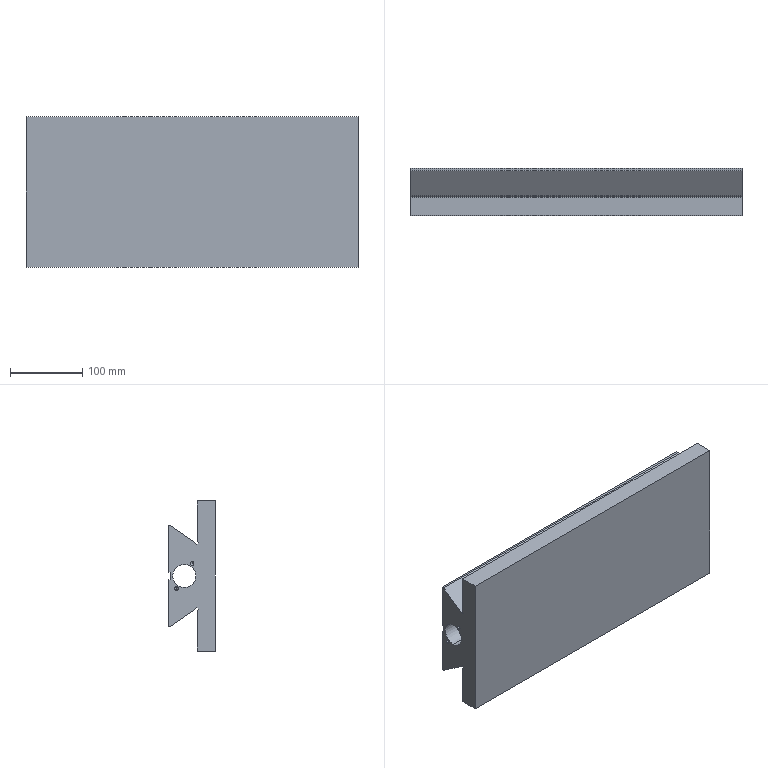Part | SolidWorks | features HoleWzd 2, ICE 2, Extrusion 1 | 1 solid | 50 faces | box 460 x 65 x 208 mm | volume 2873853 mm3 | plane 30 | cylinder 12 | cone 8 | commonest cylinder face diameters 5 x8 32 x4
STEP:
#1=CARTESIAN_POINT('',(17.,19.747,14.954));
#2=VERTEX_POINT('',#1);
#3=CARTESIAN_POINT('',(17.,19.747,19.954));
#4=VERTEX_POINT('',#3);
#5=CARTESIAN_POINT('',(17.,19.747,17.454));
#6=DIRECTION('',(-1.,0.,0.));
#7=DIRECTION('',(0.,0.,1.));
#8=AXIS2_PLACEMENT_3D('',#5,#6,#7);
#9=CIRCLE('',#8,2.5);
#10=EDGE_CURVE('',#2,#4,#9,.T.);
#11=ORIENTED_EDGE('',*,*,#10,.F.);
#12=CARTESIAN_POINT('',(0.,19.747,14.954));
#13=VERTEX_POINT('',#12);
#14=CARTESIAN_POINT('',(0.,19.747,14.954));
#15=DIRECTION('',(-1.,0.,0.));
#16=VECTOR('',#15,1000.);
#17=LINE('',#14,#16);
#18=EDGE_CURVE('',#2,#13,#17,.T.);
#19=ORIENTED_EDGE('',*,*,#18,.T.);
#20=CARTESIAN_POINT('',(0.,19.747,19.954));
#21=VERTEX_POINT('',#20);
#22=CARTESIAN_POINT('',(0.,19.747,17.454));
#23=DIRECTION('',(-1.,0.,0.));
#24=DIRECTION('',(0.,0.,1.));
#25=AXIS2_PLACEMENT_3D('',#22,#23,#24);
#26=CIRCLE('',#25,2.5);
#27=EDGE_CURVE('',#13,#21,#26,.T.);
#28=ORIENTED_EDGE('',*,*,#27,.T.);
#29=CARTESIAN_POINT('',(0.,19.747,19.954));
#30=DIRECTION('',(-1.,0.,0.));
#31=VECTOR('',#30,1000.);
#32=LINE('',#29,#31);
#33=EDGE_CURVE('',#4,#21,#32,.T.);
#34=ORIENTED_EDGE('',*,*,#33,.F.);
#35=EDGE_LOOP('',(#11,#19,#28,#34));
#36=FACE_OUTER_BOUND('',#35,.T.);
#37=CARTESIAN_POINT('',(0.,19.747,17.454));
#38=DIRECTION('',(-1.,0.,0.));
#39=DIRECTION('',(0.,0.,1.));
#40=AXIS2_PLACEMENT_3D('',#37,#38,#39);
#41=CYLINDRICAL_SURFACE('',#40,2.5);
#42=ADVANCED_FACE('',(#36),#41,.F.);
#43=CARTESIAN_POINT('',(18.502,19.747,17.454));
#44=VERTEX_POINT('',#43);
#45=CARTESIAN_POINT('',(17.,19.747,19.954));
#46=DIRECTION('',(-0.515,0.,0.8572));
#47=VECTOR('',#46,1000.);
#48=LINE('',#45,#47);
#49=EDGE_CURVE('',#44,#4,#48,.T.);
#50=ORIENTED_EDGE('',*,*,#49,.F.);
#51=CARTESIAN_POINT('',(17.,19.747,14.954));
#52=DIRECTION('',(-0.515,0.,-0.8572));
#53=VECTOR('',#52,1000.);
#54=LINE('',#51,#53);
#55=EDGE_CURVE('',#44,#2,#54,.T.);
#56=ORIENTED_EDGE('',*,*,#55,.T.);
#57=ORIENTED_EDGE('',*,*,#10,.T.);
#58=EDGE_LOOP('',(#50,#56,#57));
#59=FACE_OUTER_BOUND('',#58,.T.);
#60=CARTESIAN_POINT('',(17.,19.747,17.454));
#61=DIRECTION('',(-1.,0.,0.));
#62=DIRECTION('',(0.,0.,1.));
#63=AXIS2_PLACEMENT_3D('',#60,#61,#62);
#64=CONICAL_SURFACE('',#63,2.5,1.03);
#65=ADVANCED_FACE('',(#59),#64,.F.);
#66=CARTESIAN_POINT('',(17.,41.253,-19.954));
#67=VERTEX_POINT('',#66);
#68=CARTESIAN_POINT('',(17.,41.253,-14.954));
#69=VERTEX_POINT('',#68);
#70=CARTESIAN_POINT('',(17.,41.253,-17.454));
#71=DIRECTION('',(-1.,0.,0.));
#72=DIRECTION('',(0.,0.,1.));
#73=AXIS2_PLACEMENT_3D('',#70,#71,#72);
#74=CIRCLE('',#73,2.5);
#75=EDGE_CURVE('',#67,#69,#74,.T.);
#76=ORIENTED_EDGE('',*,*,#75,.F.);
#77=CARTESIAN_POINT('',(0.,41.253,-19.954));
#78=VERTEX_POINT('',#77);
#79=CARTESIAN_POINT('',(0.,41.253,-19.954));
#80=DIRECTION('',(-1.,0.,0.));
#81=VECTOR('',#80,1000.);
#82=LINE('',#79,#81);
#83=EDGE_CURVE('',#67,#78,#82,.T.);
#84=ORIENTED_EDGE('',*,*,#83,.T.);
#85=CARTESIAN_POINT('',(0.,41.253,-14.954));
#86=VERTEX_POINT('',#85);
#87=CARTESIAN_POINT('',(0.,41.253,-17.454));
#88=DIRECTION('',(-1.,0.,0.));
#89=DIRECTION('',(0.,0.,1.));
#90=AXIS2_PLACEMENT_3D('',#87,#88,#89);
#91=CIRCLE('',#90,2.5);
#92=EDGE_CURVE('',#78,#86,#91,.T.);
#93=ORIENTED_EDGE('',*,*,#92,.T.);
#94=CARTESIAN_POINT('',(0.,41.253,-14.954));
#95=DIRECTION('',(-1.,0.,0.));
#96=VECTOR('',#95,1000.);
#97=LINE('',#94,#96);
#98=EDGE_CURVE('',#69,#86,#97,.T.);
#99=ORIENTED_EDGE('',*,*,#98,.F.);
#100=EDGE_LOOP('',(#76,#84,#93,#99));
#101=FACE_OUTER_BOUND('',#100,.T.);
#102=CARTESIAN_POINT('',(0.,41.253,-17.454));
#103=DIRECTION('',(-1.,0.,0.));
#104=DIRECTION('',(0.,0.,1.));
#105=AXIS2_PLACEMENT_3D('',#102,#103,#104);
#106=CYLINDRICAL_SURFACE('',#105,2.5);
#107=ADVANCED_FACE('',(#101),#106,.F.);
#108=CARTESIAN_POINT('',(18.502,41.253,-17.454));
#109=VERTEX_POINT('',#108);
#110=CARTESIAN_POINT('',(17.,41.253,-14.954));
#111=DIRECTION('',(-0.515,0.,0.8572));
#112=VECTOR('',#111,1000.);
#113=LINE('',#110,#112);
#114=EDGE_CURVE('',#109,#69,#113,.T.);
#115=ORIENTED_EDGE('',*,*,#114,.F.);
#116=CARTESIAN_POINT('',(17.,41.253,-19.954));
#117=DIRECTION('',(-0.515,0.,-0.8572));
#118=VECTOR('',#117,1000.);
#119=LINE('',#116,#118);
#120=EDGE_CURVE('',#109,#67,#119,.T.);
#121=ORIENTED_EDGE('',*,*,#120,.T.);
#122=ORIENTED_EDGE('',*,*,#75,.T.);
#123=EDGE_LOOP('',(#115,#121,#122));
#124=FACE_OUTER_BOUND('',#123,.T.);
#125=CARTESIAN_POINT('',(17.,41.253,-17.454));
#126=DIRECTION('',(-1.,0.,0.));
#127=DIRECTION('',(0.,0.,1.));
#128=AXIS2_PLACEMENT_3D('',#125,#126,#127);
#129=CONICAL_SURFACE('',#128,2.5,1.03);
#130=ADVANCED_FACE('',(#124),#129,.F.);
#131=CARTESIAN_POINT('',(443.,30.5,23.));
#132=VERTEX_POINT('',#131);
#133=CARTESIAN_POINT('',(443.,30.5,18.));
#134=VERTEX_POINT('',#133);
#135=CARTESIAN_POINT('',(443.,30.5,20.5));
#136=DIRECTION('',(1.,0.,0.));
#137=DIRECTION('',(0.,0.,-1.));
#138=AXIS2_PLACEMENT_3D('',#135,#136,#137);
#139=CIRCLE('',#138,2.5);
#140=EDGE_CURVE('',#132,#134,#139,.T.);
#141=ORIENTED_EDGE('',*,*,#140,.F.);
#142=CARTESIAN_POINT('',(460.,30.5,23.));
#143=VERTEX_POINT('',#142);
#144=CARTESIAN_POINT('',(460.,30.5,23.));
#145=DIRECTION('',(1.,0.,0.));
#146=VECTOR('',#145,1000.);
#147=LINE('',#144,#146);
#148=EDGE_CURVE('',#132,#143,#147,.T.);
#149=ORIENTED_EDGE('',*,*,#148,.T.);
#150=CARTESIAN_POINT('',(460.,30.5,18.));
#151=VERTEX_POINT('',#150);
#152=CARTESIAN_POINT('',(460.,30.5,20.5));
#153=DIRECTION('',(1.,0.,0.));
#154=DIRECTION('',(0.,0.,-1.));
#155=AXIS2_PLACEMENT_3D('',#152,#153,#154);
#156=CIRCLE('',#155,2.5);
#157=EDGE_CURVE('',#143,#151,#156,.T.);
#158=ORIENTED_EDGE('',*,*,#157,.T.);
#159=CARTESIAN_POINT('',(460.,30.5,18.));
#160=DIRECTION('',(1.,0.,0.));
#161=VECTOR('',#160,1000.);
#162=LINE('',#159,#161);
#163=EDGE_CURVE('',#134,#151,#162,.T.);
#164=ORIENTED_EDGE('',*,*,#163,.F.);
#165=EDGE_LOOP('',(#141,#149,#158,#164));
#166=FACE_OUTER_BOUND('',#165,.T.);
#167=CARTESIAN_POINT('',(460.,30.5,20.5));
#168=DIRECTION('',(1.,0.,0.));
#169=DIRECTION('',(0.,0.,-1.));
#170=AXIS2_PLACEMENT_3D('',#167,#168,#169);
#171=CYLINDRICAL_SURFACE('',#170,2.5);
#172=ADVANCED_FACE('',(#166),#171,.F.);
#173=CARTESIAN_POINT('',(441.498,30.5,20.5));
#174=VERTEX_POINT('',#173);
#175=CARTESIAN_POINT('',(443.,30.5,18.));
#176=DIRECTION('',(0.515,0.,-0.8572));
#177=VECTOR('',#176,1000.);
#178=LINE('',#175,#177);
#179=EDGE_CURVE('',#174,#134,#178,.T.);
#180=ORIENTED_EDGE('',*,*,#179,.F.);
#181=CARTESIAN_POINT('',(443.,30.5,23.));
#182=DIRECTION('',(0.515,0.,0.8572));
#183=VECTOR('',#182,1000.);
#184=LINE('',#181,#183);
#185=EDGE_CURVE('',#174,#132,#184,.T.);
#186=ORIENTED_EDGE('',*,*,#185,.T.);
#187=ORIENTED_EDGE('',*,*,#140,.T.);
#188=EDGE_LOOP('',(#180,#186,#187));
#189=FACE_OUTER_BOUND('',#188,.T.);
#190=CARTESIAN_POINT('',(443.,30.5,20.5));
#191=DIRECTION('',(1.,0.,0.));
#192=DIRECTION('',(0.,0.,-1.));
#193=AXIS2_PLACEMENT_3D('',#190,#191,#192);
#194=CONICAL_SURFACE('',#193,2.5,1.03);
#195=ADVANCED_FACE('',(#189),#194,.F.);
#196=CARTESIAN_POINT('',(443.,30.5,-18.));
#197=VERTEX_POINT('',#196);
#198=CARTESIAN_POINT('',(443.,30.5,-23.));
#199=VERTEX_POINT('',#198);
#200=CARTESIAN_POINT('',(443.,30.5,-20.5));
#201=DIRECTION('',(1.,0.,0.));
#202=DIRECTION('',(0.,0.,-1.));
#203=AXIS2_PLACEMENT_3D('',#200,#201,#202);
#204=CIRCLE('',#203,2.5);
#205=EDGE_CURVE('',#197,#199,#204,.T.);
#206=ORIENTED_EDGE('',*,*,#205,.F.);
#207=CARTESIAN_POINT('',(460.,30.5,-18.));
#208=VERTEX_POINT('',#207);
#209=CARTESIAN_POINT('',(460.,30.5,-18.));
#210=DIRECTION('',(1.,0.,0.));
#211=VECTOR('',#210,1000.);
#212=LINE('',#209,#211);
#213=EDGE_CURVE('',#197,#208,#212,.T.);
#214=ORIENTED_EDGE('',*,*,#213,.T.);
#215=CARTESIAN_POINT('',(460.,30.5,-23.));
#216=VERTEX_POINT('',#215);
#217=CARTESIAN_POINT('',(460.,30.5,-20.5));
#218=DIRECTION('',(1.,0.,0.));
#219=DIRECTION('',(0.,0.,-1.));
#220=AXIS2_PLACEMENT_3D('',#217,#218,#219);
#221=CIRCLE('',#220,2.5);
#222=EDGE_CURVE('',#208,#216,#221,.T.);
#223=ORIENTED_EDGE('',*,*,#222,.T.);
#224=CARTESIAN_POINT('',(460.,30.5,-23.));
#225=DIRECTION('',(1.,0.,0.));
#226=VECTOR('',#225,1000.);
#227=LINE('',#224,#226);
#228=EDGE_CURVE('',#199,#216,#227,.T.);
#229=ORIENTED_EDGE('',*,*,#228,.F.);
#230=EDGE_LOOP('',(#206,#214,#223,#229));
#231=FACE_OUTER_BOUND('',#230,.T.);
#232=CARTESIAN_POINT('',(460.,30.5,-20.5));
#233=DIRECTION('',(1.,0.,0.));
#234=DIRECTION('',(0.,0.,-1.));
#235=AXIS2_PLACEMENT_3D('',#232,#233,#234);
#236=CYLINDRICAL_SURFACE('',#235,2.5);
#237=ADVANCED_FACE('',(#231),#236,.F.);
#238=CARTESIAN_POINT('',(441.498,30.5,-20.5));
#239=VERTEX_POINT('',#238);
#240=CARTESIAN_POINT('',(443.,30.5,-23.));
#241=DIRECTION('',(0.515,0.,-0.8572));
#242=VECTOR('',#241,1000.);
#243=LINE('',#240,#242);
#244=EDGE_CURVE('',#239,#199,#243,.T.);
#245=ORIENTED_EDGE('',*,*,#244,.F.);
#246=CARTESIAN_POINT('',(443.,30.5,-18.));
#247=DIRECTION('',(0.515,0.,0.8572));
#248=VECTOR('',#247,1000.);
#249=LINE('',#246,#248);
#250=EDGE_CURVE('',#239,#197,#249,.T.);
#251=ORIENTED_EDGE('',*,*,#250,.T.);
#252=ORIENTED_EDGE('',*,*,#205,.T.);
#253=EDGE_LOOP('',(#245,#251,#252));
#254=FACE_OUTER_BOUND('',#253,.T.);
#255=CARTESIAN_POINT('',(443.,30.5,-20.5));
#256=DIRECTION('',(1.,0.,0.));
#257=DIRECTION('',(0.,0.,-1.));
#258=AXIS2_PLACEMENT_3D('',#255,#256,#257);
#259=CONICAL_SURFACE('',#258,2.5,1.03);
#260=ADVANCED_FACE('',(#254),#259,.F.);
#261=CARTESIAN_POINT('',(430.,30.5,16.));
#262=VERTEX_POINT('',#261);
#263=CARTESIAN_POINT('',(430.,30.5,-16.));
#264=VERTEX_POINT('',#263);
#265=CARTESIAN_POINT('',(430.,30.5,0.));
#266=DIRECTION('',(1.,0.,0.));
#267=DIRECTION('',(0.,0.,-1.));
#268=AXIS2_PLACEMENT_3D('',#265,#266,#267);
#269=CIRCLE('',#268,16.);
#270=EDGE_CURVE('',#262,#264,#269,.T.);
#271=ORIENTED_EDGE('',*,*,#270,.F.);
#272=CARTESIAN_POINT('',(460.,30.5,16.));
#273=VERTEX_POINT('',#272);
#274=CARTESIAN_POINT('',(0.,30.5,16.));
#275=DIRECTION('',(1.,0.,0.));
#276=VECTOR('',#275,1000.);
#277=LINE('',#274,#276);
#278=EDGE_CURVE('',#262,#273,#277,.T.);
#279=ORIENTED_EDGE('',*,*,#278,.T.);
#280=CARTESIAN_POINT('',(460.,30.5,-16.));
#281=VERTEX_POINT('',#280);
#282=CARTESIAN_POINT('',(460.,30.5,0.));
#283=DIRECTION('',(1.,0.,0.));
#284=DIRECTION('',(0.,0.,-1.));
#285=AXIS2_PLACEMENT_3D('',#282,#283,#284);
#286=CIRCLE('',#285,16.);
#287=EDGE_CURVE('',#273,#281,#286,.T.);
#288=ORIENTED_EDGE('',*,*,#287,.T.);
#289=CARTESIAN_POINT('',(0.,30.5,-16.));
#290=DIRECTION('',(1.,0.,0.));
#291=VECTOR('',#290,1000.);
#292=LINE('',#289,#291);
#293=EDGE_CURVE('',#264,#281,#292,.T.);
#294=ORIENTED_EDGE('',*,*,#293,.F.);
#295=EDGE_LOOP('',(#271,#279,#288,#294));
#296=FACE_OUTER_BOUND('',#295,.T.);
#297=CARTESIAN_POINT('',(0.,30.5,0.));
#298=DIRECTION('',(1.,0.,0.));
#299=DIRECTION('',(0.,0.,-1.));
#300=AXIS2_PLACEMENT_3D('',#297,#298,#299);
#301=CYLINDRICAL_SURFACE('',#300,16.);
#302=ADVANCED_FACE('',(#296),#301,.F.);
#303=CARTESIAN_POINT('',(0.,30.5,16.));
#304=VERTEX_POINT('',#303);
#305=CARTESIAN_POINT('',(0.,30.5,-16.));
#306=VERTEX_POINT('',#305);
#307=CARTESIAN_POINT('',(0.,30.5,0.));
#308=DIRECTION('',(1.,0.,0.));
#309=DIRECTION('',(0.,0.,-1.));
#310=AXIS2_PLACEMENT_3D('',#307,#308,#309);
#311=CIRCLE('',#310,16.);
#312=EDGE_CURVE('',#304,#306,#311,.T.);
#313=ORIENTED_EDGE('',*,*,#312,.F.);
#314=CARTESIAN_POINT('',(30.,30.5,16.));
#315=VERTEX_POINT('',#314);
#316=CARTESIAN_POINT('',(0.,30.5,16.));
#317=DIRECTION('',(1.,0.,0.));
#318=VECTOR('',#317,1000.);
#319=LINE('',#316,#318);
#320=EDGE_CURVE('',#304,#315,#319,.T.);
#321=ORIENTED_EDGE('',*,*,#320,.T.);
#322=CARTESIAN_POINT('',(30.,30.5,-16.));
#323=VERTEX_POINT('',#322);
#324=CARTESIAN_POINT('',(30.,30.5,0.));
#325=DIRECTION('',(-1.,0.,0.));
#326=DIRECTION('',(0.,0.,1.));
#327=AXIS2_PLACEMENT_3D('',#324,#325,#326);
#328=CIRCLE('',#327,16.);
#329=EDGE_CURVE('',#323,#315,#328,.T.);
#330=ORIENTED_EDGE('',*,*,#329,.F.);
#331=CARTESIAN_POINT('',(0.,30.5,-16.));
#332=DIRECTION('',(1.,0.,0.));
#333=VECTOR('',#332,1000.);
#334=LINE('',#331,#333);
#335=EDGE_CURVE('',#306,#323,#334,.T.);
#336=ORIENTED_EDGE('',*,*,#335,.F.);
#337=EDGE_LOOP('',(#313,#321,#330,#336));
#338=FACE_OUTER_BOUND('',#337,.T.);
#339=CARTESIAN_POINT('',(0.,30.5,0.));
#340=DIRECTION('',(1.,0.,0.));
#341=DIRECTION('',(0.,0.,-1.));
#342=AXIS2_PLACEMENT_3D('',#339,#340,#341);
#343=CYLINDRICAL_SURFACE('',#342,16.);
#344=ADVANCED_FACE('',(#338),#343,.F.);
#345=CARTESIAN_POINT('',(460.,52.5,-5.));
#346=VERTEX_POINT('',#345);
#347=CARTESIAN_POINT('',(430.,52.5,-5.));
#348=VERTEX_POINT('',#347);
#349=CARTESIAN_POINT('',(460.,52.5,-5.));
#350=DIRECTION('',(-1.,0.,0.));
#351=VECTOR('',#350,1000.);
#352=LINE('',#349,#351);
#353=EDGE_CURVE('',#346,#348,#352,.T.);
#354=ORIENTED_EDGE('',*,*,#353,.T.);
#355=CARTESIAN_POINT('',(430.,49.917,-5.));
#356=VERTEX_POINT('',#355);
#357=CARTESIAN_POINT('',(430.,52.5,-5.));
#358=DIRECTION('',(0.,-1.,0.));
#359=VECTOR('',#358,1000.);
#360=LINE('',#357,#359);
#361=EDGE_CURVE('',#348,#356,#360,.T.);
#362=ORIENTED_EDGE('',*,*,#361,.T.);
#363=CARTESIAN_POINT('',(460.,49.917,-5.));
#364=VERTEX_POINT('',#363);
#365=CARTESIAN_POINT('',(460.,49.917,-5.));
#366=DIRECTION('',(-1.,0.,0.));
#367=VECTOR('',#366,1000.);
#368=LINE('',#365,#367);
#369=EDGE_CURVE('',#364,#356,#368,.T.);
#370=ORIENTED_EDGE('',*,*,#369,.F.);
#371=CARTESIAN_POINT('',(460.,52.5,-5.));
#372=DIRECTION('',(0.,-1.,0.));
#373=VECTOR('',#372,1000.);
#374=LINE('',#371,#373);
#375=EDGE_CURVE('',#346,#364,#374,.T.);
#376=ORIENTED_EDGE('',*,*,#375,.F.);
#377=EDGE_LOOP('',(#354,#362,#370,#376));
#378=FACE_OUTER_BOUND('',#377,.T.);
#379=CARTESIAN_POINT('',(460.,52.5,-5.));
#380=DIRECTION('',(0.,0.,-1.));
#381=DIRECTION('',(-1.,0.,0.));
#382=AXIS2_PLACEMENT_3D('',#379,#380,#381);
#383=PLANE('',#382);
#384=ADVANCED_FACE('',(#378),#383,.F.);
#385=ORIENTED_EDGE('',*,*,#369,.T.);
#386=CARTESIAN_POINT('',(430.,49.917,5.));
#387=VERTEX_POINT('',#386);
#388=CARTESIAN_POINT('',(430.,49.917,5.));
#389=DIRECTION('',(0.,0.,1.));
#390=VECTOR('',#389,1000.);
#391=LINE('',#388,#390);
#392=EDGE_CURVE('',#356,#387,#391,.T.);
#393=ORIENTED_EDGE('',*,*,#392,.T.);
#394=CARTESIAN_POINT('',(460.,49.917,5.));
#395=VERTEX_POINT('',#394);
#396=CARTESIAN_POINT('',(460.,49.917,5.));
#397=DIRECTION('',(-1.,0.,0.));
#398=VECTOR('',#397,1000.);
#399=LINE('',#396,#398);
#400=EDGE_CURVE('',#395,#387,#399,.T.);
#401=ORIENTED_EDGE('',*,*,#400,.F.);
#402=CARTESIAN_POINT('',(460.,49.917,5.));
#403=DIRECTION('',(0.,0.,1.));
#404=VECTOR('',#403,1000.);
#405=LINE('',#402,#404);
#406=EDGE_CURVE('',#364,#395,#405,.T.);
#407=ORIENTED_EDGE('',*,*,#406,.F.);
#408=EDGE_LOOP('',(#385,#393,#401,#407));
#409=FACE_OUTER_BOUND('',#408,.T.);
#410=CARTESIAN_POINT('',(460.,49.917,5.));
#411=DIRECTION('',(0.,-1.,0.));
#412=DIRECTION('',(0.,0.,-1.));
#413=AXIS2_PLACEMENT_3D('',#410,#411,#412);
#414=PLANE('',#413);
#415=ADVANCED_FACE('',(#409),#414,.F.);
#416=ORIENTED_EDGE('',*,*,#400,.T.);
#417=CARTESIAN_POINT('',(430.,52.5,5.));
#418=VERTEX_POINT('',#417);
#419=CARTESIAN_POINT('',(430.,52.5,5.));
#420=DIRECTION('',(0.,1.,0.));
#421=VECTOR('',#420,1000.);
#422=LINE('',#419,#421);
#423=EDGE_CURVE('',#387,#418,#422,.T.);
#424=ORIENTED_EDGE('',*,*,#423,.T.);
#425=CARTESIAN_POINT('',(460.,52.5,5.));
#426=VERTEX_POINT('',#425);
#427=CARTESIAN_POINT('',(460.,52.5,5.));
#428=DIRECTION('',(-1.,0.,0.));
#429=VECTOR('',#428,1000.);
#430=LINE('',#427,#429);
#431=EDGE_CURVE('',#426,#418,#430,.T.);
#432=ORIENTED_EDGE('',*,*,#431,.F.);
#433=CARTESIAN_POINT('',(460.,52.5,5.));
#434=DIRECTION('',(0.,1.,0.));
#435=VECTOR('',#434,1000.);
#436=LINE('',#433,#435);
#437=EDGE_CURVE('',#395,#426,#436,.T.);
#438=ORIENTED_EDGE('',*,*,#437,.F.);
#439=EDGE_LOOP('',(#416,#424,#432,#438));
#440=FACE_OUTER_BOUND('',#439,.T.);
#441=CARTESIAN_POINT('',(460.,52.5,5.));
#442=DIRECTION('',(0.,0.,1.));
#443=DIRECTION('',(1.,0.,0.));
#444=AXIS2_PLACEMENT_3D('',#441,#442,#443);
#445=PLANE('',#444);
#446=ADVANCED_FACE('',(#440),#445,.F.);
#447=CARTESIAN_POINT('',(0.,-12.5,-104.));
#448=VERTEX_POINT('',#447);
#449=CARTESIAN_POINT('',(0.,12.5,-104.));
#450=VERTEX_POINT('',#449);
#451=CARTESIAN_POINT('',(0.,12.5,-104.));
#452=DIRECTION('',(0.,1.,0.));
#453=VECTOR('',#452,1000.);
#454=LINE('',#451,#453);
#455=EDGE_CURVE('',#448,#450,#454,.T.);
#456=ORIENTED_EDGE('',*,*,#455,.T.);
#457=CARTESIAN_POINT('',(460.,12.5,-104.));
#458=VERTEX_POINT('',#457);
#459=CARTESIAN_POINT('',(460.,12.5,-104.));
#460=DIRECTION('',(-1.,0.,0.));
#461=VECTOR('',#460,1000.);
#462=LINE('',#459,#461);
#463=EDGE_CURVE('',#458,#450,#462,.T.);
#464=ORIENTED_EDGE('',*,*,#463,.F.);
#465=CARTESIAN_POINT('',(460.,-12.5,-104.));
#466=VERTEX_POINT('',#465);
#467=CARTESIAN_POINT('',(460.,12.5,-104.));
#468=DIRECTION('',(0.,1.,0.));
#469=VECTOR('',#468,1000.);
#470=LINE('',#467,#469);
#471=EDGE_CURVE('',#466,#458,#470,.T.);
#472=ORIENTED_EDGE('',*,*,#471,.F.);
#473=CARTESIAN_POINT('',(460.,-12.5,-104.));
#474=DIRECTION('',(-1.,0.,0.));
#475=VECTOR('',#474,1000.);
#476=LINE('',#473,#475);
#477=EDGE_CURVE('',#466,#448,#476,.T.);
#478=ORIENTED_EDGE('',*,*,#477,.T.);
#479=EDGE_LOOP('',(#456,#464,#472,#478));
#480=FACE_OUTER_BOUND('',#479,.T.);
#481=CARTESIAN_POINT('',(460.,12.5,-104.));
#482=DIRECTION('',(0.,0.,1.));
#483=DIRECTION('',(1.,0.,0.));
#484=AXIS2_PLACEMENT_3D('',#481,#482,#483);
#485=PLANE('',#484);
#486=ADVANCED_FACE('',(#480),#485,.F.);
#487=CARTESIAN_POINT('',(0.,12.5,-47.703));
#488=VERTEX_POINT('',#487);
#489=CARTESIAN_POINT('',(0.,12.5,-47.703));
#490=DIRECTION('',(0.,0.,1.));
#491=VECTOR('',#490,1000.);
#492=LINE('',#489,#491);
#493=EDGE_CURVE('',#450,#488,#492,.T.);
#494=ORIENTED_EDGE('',*,*,#493,.T.);
#495=CARTESIAN_POINT('',(460.,12.5,-47.703));
#496=VERTEX_POINT('',#495);
#497=CARTESIAN_POINT('',(460.,12.5,-47.703));
#498=DIRECTION('',(-1.,0.,0.));
#499=VECTOR('',#498,1000.);
#500=LINE('',#497,#499);
#501=EDGE_CURVE('',#496,#488,#500,.T.);
#502=ORIENTED_EDGE('',*,*,#501,.F.);
#503=CARTESIAN_POINT('',(460.,12.5,-47.703));
#504=DIRECTION('',(0.,0.,1.));
#505=VECTOR('',#504,1000.);
#506=LINE('',#503,#505);
#507=EDGE_CURVE('',#458,#496,#506,.T.);
#508=ORIENTED_EDGE('',*,*,#507,.F.);
#509=ORIENTED_EDGE('',*,*,#463,.T.);
#510=EDGE_LOOP('',(#494,#502,#508,#509));
#511=FACE_OUTER_BOUND('',#510,.T.);
#512=CARTESIAN_POINT('',(460.,12.5,-47.703));
#513=DIRECTION('',(0.,-1.,0.));
#514=DIRECTION('',(0.,0.,-1.));
#515=AXIS2_PLACEMENT_3D('',#512,#513,#514);
#516=PLANE('',#515);
#517=ADVANCED_FACE('',(#511),#516,.F.);
#518=CARTESIAN_POINT('',(0.,11.077,-46.298));
#519=VERTEX_POINT('',#518);
#520=CARTESIAN_POINT('',(0.,12.5,-47.703));
#521=DIRECTION('',(0.,-0.7115,0.7026));
#522=VECTOR('',#521,1000.);
#523=LINE('',#520,#522);
#524=EDGE_CURVE('',#488,#519,#523,.T.);
#525=ORIENTED_EDGE('',*,*,#524,.T.);
#526=CARTESIAN_POINT('',(460.,11.077,-46.298));
#527=VERTEX_POINT('',#526);
#528=CARTESIAN_POINT('',(460.,11.077,-46.298));
#529=DIRECTION('',(-1.,0.,0.));
#530=VECTOR('',#529,1000.);
#531=LINE('',#528,#530);
#532=EDGE_CURVE('',#527,#519,#531,.T.);
#533=ORIENTED_EDGE('',*,*,#532,.F.);
#534=CARTESIAN_POINT('',(460.,12.5,-47.703));
#535=DIRECTION('',(0.,-0.7115,0.7026));
#536=VECTOR('',#535,1000.);
#537=LINE('',#534,#536);
#538=EDGE_CURVE('',#496,#527,#537,.T.);
#539=ORIENTED_EDGE('',*,*,#538,.F.);
#540=ORIENTED_EDGE('',*,*,#501,.T.);
#541=EDGE_LOOP('',(#525,#533,#539,#540));
#542=FACE_OUTER_BOUND('',#541,.T.);
#543=CARTESIAN_POINT('',(460.,12.5,-47.703));
#544=DIRECTION('',(0.,-0.7026,-0.7115));
#545=DIRECTION('',(0.,0.7115,-0.7026));
#546=AXIS2_PLACEMENT_3D('',#543,#544,#545);
#547=PLANE('',#546);
#548=ADVANCED_FACE('',(#542),#547,.F.);
#549=CARTESIAN_POINT('',(0.,13.185,-44.163));
#550=VERTEX_POINT('',#549);
#551=CARTESIAN_POINT('',(0.,11.077,-46.298));
#552=DIRECTION('',(0.,0.7026,0.7115));
#553=VECTOR('',#552,1000.);
#554=LINE('',#551,#553);
#555=EDGE_CURVE('',#519,#550,#554,.T.);
#556=ORIENTED_EDGE('',*,*,#555,.T.);
#557=CARTESIAN_POINT('',(460.,13.185,-44.163));
#558=VERTEX_POINT('',#557);
#559=CARTESIAN_POINT('',(460.,13.185,-44.163));
#560=DIRECTION('',(-1.,0.,0.));
#561=VECTOR('',#560,1000.);
#562=LINE('',#559,#561);
#563=EDGE_CURVE('',#558,#550,#562,.T.);
#564=ORIENTED_EDGE('',*,*,#563,.F.);
#565=CARTESIAN_POINT('',(460.,11.077,-46.298));
#566=DIRECTION('',(0.,0.7026,0.7115));
#567=VECTOR('',#566,1000.);
#568=LINE('',#565,#567);
#569=EDGE_CURVE('',#527,#558,#568,.T.);
#570=ORIENTED_EDGE('',*,*,#569,.F.);
#571=ORIENTED_EDGE('',*,*,#532,.T.);
#572=EDGE_LOOP('',(#556,#564,#570,#571));
#573=FACE_OUTER_BOUND('',#572,.T.);
#574=CARTESIAN_POINT('',(460.,11.077,-46.298));
#575=DIRECTION('',(0.,-0.7115,0.7026));
#576=DIRECTION('',(0.,-0.7026,-0.7115));
#577=AXIS2_PLACEMENT_3D('',#574,#575,#576);
#578=PLANE('',#577);
#579=ADVANCED_FACE('',(#573),#578,.F.);
#580=CARTESIAN_POINT('',(0.,14.608,-45.568));
#581=VERTEX_POINT('',#580);
#582=CARTESIAN_POINT('',(0.,13.185,-44.163));
#583=DIRECTION('',(0.,0.7115,-0.7026));
#584=VECTOR('',#583,1000.);
#585=LINE('',#582,#584);
#586=EDGE_CURVE('',#550,#581,#585,.T.);
#587=ORIENTED_EDGE('',*,*,#586,.T.);
#588=CARTESIAN_POINT('',(460.,14.608,-45.568));
#589=VERTEX_POINT('',#588);
#590=CARTESIAN_POINT('',(460.,14.608,-45.568));
#591=DIRECTION('',(-1.,0.,0.));
#592=VECTOR('',#591,1000.);
#593=LINE('',#590,#592);
#594=EDGE_CURVE('',#589,#581,#593,.T.);
#595=ORIENTED_EDGE('',*,*,#594,.F.);
#596=CARTESIAN_POINT('',(460.,13.185,-44.163));
#597=DIRECTION('',(0.,0.7115,-0.7026));
#598=VECTOR('',#597,1000.);
#599=LINE('',#596,#598);
#600=EDGE_CURVE('',#558,#589,#599,.T.);
#601=ORIENTED_EDGE('',*,*,#600,.F.);
#602=ORIENTED_EDGE('',*,*,#563,.T.);
#603=EDGE_LOOP('',(#587,#595,#601,#602));
#604=FACE_OUTER_BOUND('',#603,.T.);
#605=CARTESIAN_POINT('',(460.,13.185,-44.163));
#606=DIRECTION('',(0.,0.7026,0.7115));
#607=DIRECTION('',(0.,-0.7115,0.7026));
#608=AXIS2_PLACEMENT_3D('',#605,#606,#607);
#609=PLANE('',#608);
#610=ADVANCED_FACE('',(#604),#609,.F.);
#611=CARTESIAN_POINT('',(0.,49.5,-70.));
#612=VERTEX_POINT('',#611);
#613=CARTESIAN_POINT('',(0.,14.608,-45.568));
#614=DIRECTION('',(0.,0.8192,-0.5736));
#615=VECTOR('',#614,1000.);
#616=LINE('',#613,#615);
#617=EDGE_CURVE('',#581,#612,#616,.T.);
#618=ORIENTED_EDGE('',*,*,#617,.T.);
#619=CARTESIAN_POINT('',(460.,49.5,-70.));
#620=VERTEX_POINT('',#619);
#621=CARTESIAN_POINT('',(460.,49.5,-70.));
#622=DIRECTION('',(-1.,0.,0.));
#623=VECTOR('',#622,1000.);
#624=LINE('',#621,#623);
#625=EDGE_CURVE('',#620,#612,#624,.T.);
#626=ORIENTED_EDGE('',*,*,#625,.F.);
#627=CARTESIAN_POINT('',(460.,14.608,-45.568));
#628=DIRECTION('',(0.,0.8192,-0.5736));
#629=VECTOR('',#628,1000.);
#630=LINE('',#627,#629);
#631=EDGE_CURVE('',#589,#620,#630,.T.);
#632=ORIENTED_EDGE('',*,*,#631,.F.);
#633=ORIENTED_EDGE('',*,*,#594,.T.);
#634=EDGE_LOOP('',(#618,#626,#632,#633));
#635=FACE_OUTER_BOUND('',#634,.T.);
#636=CARTESIAN_POINT('',(460.,14.608,-45.568));
#637=DIRECTION('',(0.,0.5736,0.8192));
#638=DIRECTION('',(0.,-0.8192,0.5736));
#639=AXIS2_PLACEMENT_3D('',#636,#637,#638);
#640=PLANE('',#639);
#641=ADVANCED_FACE('',(#635),#640,.F.);
#642=CARTESIAN_POINT('',(0.,52.5,-70.));
#643=VERTEX_POINT('',#642);
#644=CARTESIAN_POINT('',(0.,52.5,-70.));
#645=DIRECTION('',(0.,1.,0.));
#646=VECTOR('',#645,1000.);
#647=LINE('',#644,#646);
#648=EDGE_CURVE('',#612,#643,#647,.T.);
#649=ORIENTED_EDGE('',*,*,#648,.T.);
#650=CARTESIAN_POINT('',(460.,52.5,-70.));
#651=VERTEX_POINT('',#650);
#652=CARTESIAN_POINT('',(460.,52.5,-70.));
#653=DIRECTION('',(-1.,0.,0.));
#654=VECTOR('',#653,1000.);
#655=LINE('',#652,#654);
#656=EDGE_CURVE('',#651,#643,#655,.T.);
#657=ORIENTED_EDGE('',*,*,#656,.F.);
#658=CARTESIAN_POINT('',(460.,52.5,-70.));
#659=DIRECTION('',(0.,1.,0.));
#660=VECTOR('',#659,1000.);
#661=LINE('',#658,#660);
#662=EDGE_CURVE('',#620,#651,#661,.T.);
#663=ORIENTED_EDGE('',*,*,#662,.F.);
#664=ORIENTED_EDGE('',*,*,#625,.T.);
#665=EDGE_LOOP('',(#649,#657,#663,#664));
#666=FACE_OUTER_BOUND('',#665,.T.);
#667=CARTESIAN_POINT('',(460.,52.5,-70.));
#668=DIRECTION('',(0.,0.,1.));
#669=DIRECTION('',(1.,0.,0.));
#670=AXIS2_PLACEMENT_3D('',#667,#668,#669);
#671=PLANE('',#670);
#672=ADVANCED_FACE('',(#666),#671,.F.);
#673=CARTESIAN_POINT('',(430.,52.5,-40.));
#674=VERTEX_POINT('',#673);
#675=CARTESIAN_POINT('',(30.,52.5,-40.));
#676=VERTEX_POINT('',#675);
#677=CARTESIAN_POINT('',(30.,52.5,-40.));
#678=DIRECTION('',(-1.,0.,0.));
#679=VECTOR('',#678,1000.);
#680=LINE('',#677,#679);
#681=EDGE_CURVE('',#674,#676,#680,.T.);
#682=ORIENTED_EDGE('',*,*,#681,.F.);
#683=CARTESIAN_POINT('',(430.,52.5,-40.));
#684=DIRECTION('',(0.,0.,-1.));
#685=VECTOR('',#684,1000.);
#686=LINE('',#683,#685);
#687=EDGE_CURVE('',#348,#674,#686,.T.);
#688=ORIENTED_EDGE('',*,*,#687,.F.);
#689=ORIENTED_EDGE('',*,*,#353,.F.);
#690=CARTESIAN_POINT('',(460.,52.5,-70.));
#691=DIRECTION('',(0.,0.,1.));
#692=VECTOR('',#691,1000.);
#693=LINE('',#690,#692);
#694=EDGE_CURVE('',#651,#346,#693,.T.);
#695=ORIENTED_EDGE('',*,*,#694,.F.);
#696=ORIENTED_EDGE('',*,*,#656,.T.);
#697=CARTESIAN_POINT('',(0.,52.5,-5.));
#698=VERTEX_POINT('',#697);
#699=CARTESIAN_POINT('',(0.,52.5,-70.));
#700=DIRECTION('',(0.,0.,1.));
#701=VECTOR('',#700,1000.);
#702=LINE('',#699,#701);
#703=EDGE_CURVE('',#643,#698,#702,.T.);
#704=ORIENTED_EDGE('',*,*,#703,.T.);
#705=CARTESIAN_POINT('',(30.,52.5,-5.));
#706=VERTEX_POINT('',#705);
#707=CARTESIAN_POINT('',(460.,52.5,-5.));
#708=DIRECTION('',(-1.,0.,0.));
#709=VECTOR('',#708,1000.);
#710=LINE('',#707,#709);
#711=EDGE_CURVE('',#706,#698,#710,.T.);
#712=ORIENTED_EDGE('',*,*,#711,.F.);
#713=CARTESIAN_POINT('',(30.,52.5,-40.));
#714=DIRECTION('',(0.,0.,1.));
#715=VECTOR('',#714,1000.);
#716=LINE('',#713,#715);
#717=EDGE_CURVE('',#676,#706,#716,.T.);
#718=ORIENTED_EDGE('',*,*,#717,.F.);
#719=EDGE_LOOP('',(#682,#688,#689,#695,#696,#704,#712,#718));
#720=FACE_OUTER_BOUND('',#719,.T.);
#721=CARTESIAN_POINT('',(460.,52.5,-70.));
#722=DIRECTION('',(0.,-1.,0.));
#723=DIRECTION('',(0.,0.,-1.));
#724=AXIS2_PLACEMENT_3D('',#721,#722,#723);
#725=PLANE('',#724);
#726=ADVANCED_FACE('',(#720),#725,.F.);
#727=CARTESIAN_POINT('',(30.,49.917,-5.));
#728=VERTEX_POINT('',#727);
#729=CARTESIAN_POINT('',(0.,49.917,-5.));
#730=VERTEX_POINT('',#729);
#731=CARTESIAN_POINT('',(460.,49.917,-5.));
#732=DIRECTION('',(-1.,0.,0.));
#733=VECTOR('',#732,1000.);
#734=LINE('',#731,#733);
#735=EDGE_CURVE('',#728,#730,#734,.T.);
#736=ORIENTED_EDGE('',*,*,#735,.F.);
#737=CARTESIAN_POINT('',(30.,52.5,-5.));
#738=DIRECTION('',(0.,1.,0.));
#739=VECTOR('',#738,1000.);
#740=LINE('',#737,#739);
#741=EDGE_CURVE('',#728,#706,#740,.T.);
#742=ORIENTED_EDGE('',*,*,#741,.T.);
#743=ORIENTED_EDGE('',*,*,#711,.T.);
#744=CARTESIAN_POINT('',(0.,52.5,-5.));
#745=DIRECTION('',(0.,-1.,0.));
#746=VECTOR('',#745,1000.);
#747=LINE('',#744,#746);
#748=EDGE_CURVE('',#698,#730,#747,.T.);
#749=ORIENTED_EDGE('',*,*,#748,.T.);
#750=EDGE_LOOP('',(#736,#742,#743,#749));
#751=FACE_OUTER_BOUND('',#750,.T.);
#752=CARTESIAN_POINT('',(460.,52.5,-5.));
#753=DIRECTION('',(0.,0.,-1.));
#754=DIRECTION('',(-1.,0.,0.));
#755=AXIS2_PLACEMENT_3D('',#752,#753,#754);
#756=PLANE('',#755);
#757=ADVANCED_FACE('',(#751),#756,.F.);
#758=CARTESIAN_POINT('',(30.,49.917,5.));
#759=VERTEX_POINT('',#758);
#760=CARTESIAN_POINT('',(0.,49.917,5.));
#761=VERTEX_POINT('',#760);
#762=CARTESIAN_POINT('',(460.,49.917,5.));
#763=DIRECTION('',(-1.,0.,0.));
#764=VECTOR('',#763,1000.);
#765=LINE('',#762,#764);
#766=EDGE_CURVE('',#759,#761,#765,.T.);
#767=ORIENTED_EDGE('',*,*,#766,.F.);
#768=CARTESIAN_POINT('',(30.,49.917,5.));
#769=DIRECTION('',(0.,0.,-1.));
#770=VECTOR('',#769,1000.);
#771=LINE('',#768,#770);
#772=EDGE_CURVE('',#759,#728,#771,.T.);
#773=ORIENTED_EDGE('',*,*,#772,.T.);
#774=ORIENTED_EDGE('',*,*,#735,.T.);
#775=CARTESIAN_POINT('',(0.,49.917,5.));
#776=DIRECTION('',(0.,0.,1.));
#777=VECTOR('',#776,1000.);
#778=LINE('',#775,#777);
#779=EDGE_CURVE('',#730,#761,#778,.T.);
#780=ORIENTED_EDGE('',*,*,#779,.T.);
#781=EDGE_LOOP('',(#767,#773,#774,#780));
#782=FACE_OUTER_BOUND('',#781,.T.);
#783=CARTESIAN_POINT('',(460.,49.917,5.));
#784=DIRECTION('',(0.,-1.,0.));
#785=DIRECTION('',(0.,0.,-1.));
#786=AXIS2_PLACEMENT_3D('',#783,#784,#785);
#787=PLANE('',#786);
#788=ADVANCED_FACE('',(#782),#787,.F.);
#789=CARTESIAN_POINT('',(30.,52.5,5.));
#790=VERTEX_POINT('',#789);
#791=CARTESIAN_POINT('',(0.,52.5,5.));
#792=VERTEX_POINT('',#791);
#793=CARTESIAN_POINT('',(460.,52.5,5.));
#794=DIRECTION('',(-1.,0.,0.));
#795=VECTOR('',#794,1000.);
#796=LINE('',#793,#795);
#797=EDGE_CURVE('',#790,#792,#796,.T.);
#798=ORIENTED_EDGE('',*,*,#797,.F.);
#799=CARTESIAN_POINT('',(30.,52.5,5.));
#800=DIRECTION('',(0.,-1.,0.));
#801=VECTOR('',#800,1000.);
#802=LINE('',#799,#801);
#803=EDGE_CURVE('',#790,#759,#802,.T.);
#804=ORIENTED_EDGE('',*,*,#803,.T.);
#805=ORIENTED_EDGE('',*,*,#766,.T.);
#806=CARTESIAN_POINT('',(0.,52.5,5.));
#807=DIRECTION('',(0.,1.,0.));
#808=VECTOR('',#807,1000.);
#809=LINE('',#806,#808);
#810=EDGE_CURVE('',#761,#792,#809,.T.);
#811=ORIENTED_EDGE('',*,*,#810,.T.);
#812=EDGE_LOOP('',(#798,#804,#805,#811));
#813=FACE_OUTER_BOUND('',#812,.T.);
#814=CARTESIAN_POINT('',(460.,52.5,5.));
#815=DIRECTION('',(0.,0.,1.));
#816=DIRECTION('',(1.,0.,0.));
#817=AXIS2_PLACEMENT_3D('',#814,#815,#816);
#818=PLANE('',#817);
#819=ADVANCED_FACE('',(#813),#818,.F.);
#820=ORIENTED_EDGE('',*,*,#431,.T.);
#821=CARTESIAN_POINT('',(430.,52.5,40.));
#822=VERTEX_POINT('',#821);
#823=CARTESIAN_POINT('',(430.,52.5,-40.));
#824=DIRECTION('',(0.,0.,-1.));
#825=VECTOR('',#824,1000.);
#826=LINE('',#823,#825);
#827=EDGE_CURVE('',#822,#418,#826,.T.);
#828=ORIENTED_EDGE('',*,*,#827,.F.);
#829=CARTESIAN_POINT('',(30.,52.5,40.));
#830=VERTEX_POINT('',#829);
#831=CARTESIAN_POINT('',(30.,52.5,40.));
#832=DIRECTION('',(1.,0.,0.));
#833=VECTOR('',#832,1000.);
#834=LINE('',#831,#833);
#835=EDGE_CURVE('',#830,#822,#834,.T.);
#836=ORIENTED_EDGE('',*,*,#835,.F.);
#837=CARTESIAN_POINT('',(30.,52.5,70.));
#838=DIRECTION('',(0.,0.,-1.));
#839=VECTOR('',#838,1000.);
#840=LINE('',#837,#839);
#841=EDGE_CURVE('',#830,#790,#840,.T.);
#842=ORIENTED_EDGE('',*,*,#841,.T.);
#843=ORIENTED_EDGE('',*,*,#797,.T.);
#844=CARTESIAN_POINT('',(0.,52.5,70.));
#845=VERTEX_POINT('',#844);
#846=CARTESIAN_POINT('',(0.,52.5,70.));
#847=DIRECTION('',(0.,0.,1.));
#848=VECTOR('',#847,1000.);
#849=LINE('',#846,#848);
#850=EDGE_CURVE('',#792,#845,#849,.T.);
#851=ORIENTED_EDGE('',*,*,#850,.T.);
#852=CARTESIAN_POINT('',(460.,52.5,70.));
#853=VERTEX_POINT('',#852);
#854=CARTESIAN_POINT('',(460.,52.5,70.));
#855=DIRECTION('',(-1.,0.,0.));
#856=VECTOR('',#855,1000.);
#857=LINE('',#854,#856);
#858=EDGE_CURVE('',#853,#845,#857,.T.);
#859=ORIENTED_EDGE('',*,*,#858,.F.);
#860=CARTESIAN_POINT('',(460.,52.5,70.));
#861=DIRECTION('',(0.,0.,1.));
#862=VECTOR('',#861,1000.);
#863=LINE('',#860,#862);
#864=EDGE_CURVE('',#426,#853,#863,.T.);
#865=ORIENTED_EDGE('',*,*,#864,.F.);
#866=EDGE_LOOP('',(#820,#828,#836,#842,#843,#851,#859,#865));
#867=FACE_OUTER_BOUND('',#866,.T.);
#868=CARTESIAN_POINT('',(460.,52.5,70.));
#869=DIRECTION('',(0.,-1.,0.));
#870=DIRECTION('',(0.,0.,-1.));
#871=AXIS2_PLACEMENT_3D('',#868,#869,#870);
#872=PLANE('',#871);
#873=ADVANCED_FACE('',(#867),#872,.F.);
#874=CARTESIAN_POINT('',(0.,49.5,70.));
#875=VERTEX_POINT('',#874);
#876=CARTESIAN_POINT('',(0.,52.5,70.));
#877=DIRECTION('',(0.,-1.,0.));
#878=VECTOR('',#877,1000.);
#879=LINE('',#876,#878);
#880=EDGE_CURVE('',#845,#875,#879,.T.);
#881=ORIENTED_EDGE('',*,*,#880,.T.);
#882=CARTESIAN_POINT('',(460.,49.5,70.));
#883=VERTEX_POINT('',#882);
#884=CARTESIAN_POINT('',(460.,49.5,70.));
#885=DIRECTION('',(-1.,0.,0.));
#886=VECTOR('',#885,1000.);
#887=LINE('',#884,#886);
#888=EDGE_CURVE('',#883,#875,#887,.T.);
#889=ORIENTED_EDGE('',*,*,#888,.F.);
#890=CARTESIAN_POINT('',(460.,52.5,70.));
#891=DIRECTION('',(0.,-1.,0.));
#892=VECTOR('',#891,1000.);
#893=LINE('',#890,#892);
#894=EDGE_CURVE('',#853,#883,#893,.T.);
#895=ORIENTED_EDGE('',*,*,#894,.F.);
#896=ORIENTED_EDGE('',*,*,#858,.T.);
#897=EDGE_LOOP('',(#881,#889,#895,#896));
#898=FACE_OUTER_BOUND('',#897,.T.);
#899=CARTESIAN_POINT('',(460.,52.5,70.));
#900=DIRECTION('',(0.,0.,-1.));
#901=DIRECTION('',(-1.,0.,0.));
#902=AXIS2_PLACEMENT_3D('',#899,#900,#901);
#903=PLANE('',#902);
#904=ADVANCED_FACE('',(#898),#903,.F.);
#905=CARTESIAN_POINT('',(0.,14.608,45.568));
#906=VERTEX_POINT('',#905);
#907=CARTESIAN_POINT('',(0.,14.608,45.568));
#908=DIRECTION('',(0.,-0.8192,-0.5736));
#909=VECTOR('',#908,1000.);
#910=LINE('',#907,#909);
#911=EDGE_CURVE('',#875,#906,#910,.T.);
#912=ORIENTED_EDGE('',*,*,#911,.T.);
#913=CARTESIAN_POINT('',(460.,14.608,45.568));
#914=VERTEX_POINT('',#913);
#915=CARTESIAN_POINT('',(460.,14.608,45.568));
#916=DIRECTION('',(-1.,0.,0.));
#917=VECTOR('',#916,1000.);
#918=LINE('',#915,#917);
#919=EDGE_CURVE('',#914,#906,#918,.T.);
#920=ORIENTED_EDGE('',*,*,#919,.F.);
#921=CARTESIAN_POINT('',(460.,14.608,45.568));
#922=DIRECTION('',(0.,-0.8192,-0.5736));
#923=VECTOR('',#922,1000.);
#924=LINE('',#921,#923);
#925=EDGE_CURVE('',#883,#914,#924,.T.);
#926=ORIENTED_EDGE('',*,*,#925,.F.);
#927=ORIENTED_EDGE('',*,*,#888,.T.);
#928=EDGE_LOOP('',(#912,#920,#926,#927));
#929=FACE_OUTER_BOUND('',#928,.T.);
#930=CARTESIAN_POINT('',(460.,14.608,45.568));
#931=DIRECTION('',(0.,0.5736,-0.8192));
#932=DIRECTION('',(0.,0.8192,0.5736));
#933=AXIS2_PLACEMENT_3D('',#930,#931,#932);
#934=PLANE('',#933);
#935=ADVANCED_FACE('',(#929),#934,.F.);
#936=CARTESIAN_POINT('',(0.,13.185,44.163));
#937=VERTEX_POINT('',#936);
#938=CARTESIAN_POINT('',(0.,13.185,44.163));
#939=DIRECTION('',(0.,-0.7115,-0.7026));
#940=VECTOR('',#939,1000.);
#941=LINE('',#938,#940);
#942=EDGE_CURVE('',#906,#937,#941,.T.);
#943=ORIENTED_EDGE('',*,*,#942,.T.);
#944=CARTESIAN_POINT('',(460.,13.185,44.163));
#945=VERTEX_POINT('',#944);
#946=CARTESIAN_POINT('',(460.,13.185,44.163));
#947=DIRECTION('',(-1.,0.,0.));
#948=VECTOR('',#947,1000.);
#949=LINE('',#946,#948);
#950=EDGE_CURVE('',#945,#937,#949,.T.);
#951=ORIENTED_EDGE('',*,*,#950,.F.);
#952=CARTESIAN_POINT('',(460.,13.185,44.163));
#953=DIRECTION('',(0.,-0.7115,-0.7026));
#954=VECTOR('',#953,1000.);
#955=LINE('',#952,#954);
#956=EDGE_CURVE('',#914,#945,#955,.T.);
#957=ORIENTED_EDGE('',*,*,#956,.F.);
#958=ORIENTED_EDGE('',*,*,#919,.T.);
#959=EDGE_LOOP('',(#943,#951,#957,#958));
#960=FACE_OUTER_BOUND('',#959,.T.);
#961=CARTESIAN_POINT('',(460.,13.185,44.163));
#962=DIRECTION('',(0.,0.7026,-0.7115));
#963=DIRECTION('',(0.,0.7115,0.7026));
#964=AXIS2_PLACEMENT_3D('',#961,#962,#963);
#965=PLANE('',#964);
#966=ADVANCED_FACE('',(#960),#965,.F.);
#967=CARTESIAN_POINT('',(0.,11.077,46.298));
#968=VERTEX_POINT('',#967);
#969=CARTESIAN_POINT('',(0.,11.077,46.298));
#970=DIRECTION('',(0.,-0.7026,0.7115));
#971=VECTOR('',#970,1000.);
#972=LINE('',#969,#971);
#973=EDGE_CURVE('',#937,#968,#972,.T.);
#974=ORIENTED_EDGE('',*,*,#973,.T.);
#975=CARTESIAN_POINT('',(460.,11.077,46.298));
#976=VERTEX_POINT('',#975);
#977=CARTESIAN_POINT('',(460.,11.077,46.298));
#978=DIRECTION('',(-1.,0.,0.));
#979=VECTOR('',#978,1000.);
#980=LINE('',#977,#979);
#981=EDGE_CURVE('',#976,#968,#980,.T.);
#982=ORIENTED_EDGE('',*,*,#981,.F.);
#983=CARTESIAN_POINT('',(460.,11.077,46.298));
#984=DIRECTION('',(0.,-0.7026,0.7115));
#985=VECTOR('',#984,1000.);
#986=LINE('',#983,#985);
#987=EDGE_CURVE('',#945,#976,#986,.T.);
#988=ORIENTED_EDGE('',*,*,#987,.F.);
#989=ORIENTED_EDGE('',*,*,#950,.T.);
#990=EDGE_LOOP('',(#974,#982,#988,#989));
#991=FACE_OUTER_BOUND('',#990,.T.);
#992=CARTESIAN_POINT('',(460.,11.077,46.298));
#993=DIRECTION('',(0.,-0.7115,-0.7026));
#994=DIRECTION('',(0.,0.7026,-0.7115));
#995=AXIS2_PLACEMENT_3D('',#992,#993,#994);
#996=PLANE('',#995);
#997=ADVANCED_FACE('',(#991),#996,.F.);
#998=CARTESIAN_POINT('',(0.,12.5,47.703));
#999=VERTEX_POINT('',#998);
#1000=CARTESIAN_POINT('',(0.,12.5,47.703));
#1001=DIRECTION('',(0.,0.7115,0.7026));
#1002=VECTOR('',#1001,1000.);
#1003=LINE('',#1000,#1002);
#1004=EDGE_CURVE('',#968,#999,#1003,.T.);
#1005=ORIENTED_EDGE('',*,*,#1004,.T.);
#1006=CARTESIAN_POINT('',(460.,12.5,47.703));
#1007=VERTEX_POINT('',#1006);
#1008=CARTESIAN_POINT('',(460.,12.5,47.703));
#1009=DIRECTION('',(-1.,0.,0.));
#1010=VECTOR('',#1009,1000.);
#1011=LINE('',#1008,#1010);
#1012=EDGE_CURVE('',#1007,#999,#1011,.T.);
#1013=ORIENTED_EDGE('',*,*,#1012,.F.);
#1014=CARTESIAN_POINT('',(460.,12.5,47.703));
#1015=DIRECTION('',(0.,0.7115,0.7026));
#1016=VECTOR('',#1015,1000.);
#1017=LINE('',#1014,#1016);
#1018=EDGE_CURVE('',#976,#1007,#1017,.T.);
#1019=ORIENTED_EDGE('',*,*,#1018,.F.);
#1020=ORIENTED_EDGE('',*,*,#981,.T.);
#1021=EDGE_LOOP('',(#1005,#1013,#1019,#1020));
#1022=FACE_OUTER_BOUND('',#1021,.T.);
#1023=CARTESIAN_POINT('',(460.,12.5,47.703));
#1024=DIRECTION('',(0.,-0.7026,0.7115));
#1025=DIRECTION('',(0.,-0.7115,-0.7026));
#1026=AXIS2_PLACEMENT_3D('',#1023,#1024,#1025);
#1027=PLANE('',#1026);
#1028=ADVANCED_FACE('',(#1022),#1027,.F.);
#1029=CARTESIAN_POINT('',(0.,12.5,104.));
#1030=VERTEX_POINT('',#1029);
#1031=CARTESIAN_POINT('',(0.,12.5,104.));
#1032=DIRECTION('',(0.,0.,1.));
#1033=VECTOR('',#1032,1000.);
#1034=LINE('',#1031,#1033);
#1035=EDGE_CURVE('',#999,#1030,#1034,.T.);
#1036=ORIENTED_EDGE('',*,*,#1035,.T.);
#1037=CARTESIAN_POINT('',(460.,12.5,104.));
#1038=VERTEX_POINT('',#1037);
#1039=CARTESIAN_POINT('',(460.,12.5,104.));
#1040=DIRECTION('',(-1.,0.,0.));
#1041=VECTOR('',#1040,1000.);
#1042=LINE('',#1039,#1041);
#1043=EDGE_CURVE('',#1038,#1030,#1042,.T.);
#1044=ORIENTED_EDGE('',*,*,#1043,.F.);
#1045=CARTESIAN_POINT('',(460.,12.5,104.));
#1046=DIRECTION('',(0.,0.,1.));
#1047=VECTOR('',#1046,1000.);
#1048=LINE('',#1045,#1047);
#1049=EDGE_CURVE('',#1007,#1038,#1048,.T.);
#1050=ORIENTED_EDGE('',*,*,#1049,.F.);
#1051=ORIENTED_EDGE('',*,*,#1012,.T.);
#1052=EDGE_LOOP('',(#1036,#1044,#1050,#1051));
#1053=FACE_OUTER_BOUND('',#1052,.T.);
#1054=CARTESIAN_POINT('',(460.,12.5,104.));
#1055=DIRECTION('',(0.,-1.,0.));
#1056=DIRECTION('',(0.,0.,-1.));
#1057=AXIS2_PLACEMENT_3D('',#1054,#1055,#1056);
#1058=PLANE('',#1057);
#1059=ADVANCED_FACE('',(#1053),#1058,.F.);
#1060=CARTESIAN_POINT('',(0.,-12.5,104.));
#1061=VERTEX_POINT('',#1060);
#1062=CARTESIAN_POINT('',(0.,12.5,104.));
#1063=DIRECTION('',(0.,-1.,0.));
#1064=VECTOR('',#1063,1000.);
#1065=LINE('',#1062,#1064);
#1066=EDGE_CURVE('',#1030,#1061,#1065,.T.);
#1067=ORIENTED_EDGE('',*,*,#1066,.T.);
#1068=CARTESIAN_POINT('',(460.,-12.5,104.));
#1069=VERTEX_POINT('',#1068);
#1070=CARTESIAN_POINT('',(460.,-12.5,104.));
#1071=DIRECTION('',(-1.,0.,0.));
#1072=VECTOR('',#1071,1000.);
#1073=LINE('',#1070,#1072);
#1074=EDGE_CURVE('',#1069,#1061,#1073,.T.);
#1075=ORIENTED_EDGE('',*,*,#1074,.F.);
#1076=CARTESIAN_POINT('',(460.,12.5,104.));
#1077=DIRECTION('',(0.,-1.,0.));
#1078=VECTOR('',#1077,1000.);
#1079=LINE('',#1076,#1078);
#1080=EDGE_CURVE('',#1038,#1069,#1079,.T.);
#1081=ORIENTED_EDGE('',*,*,#1080,.F.);
#1082=ORIENTED_EDGE('',*,*,#1043,.T.);
#1083=EDGE_LOOP('',(#1067,#1075,#1081,#1082));
#1084=FACE_OUTER_BOUND('',#1083,.T.);
#1085=CARTESIAN_POINT('',(460.,12.5,104.));
#1086=DIRECTION('',(0.,0.,-1.));
#1087=DIRECTION('',(-1.,0.,0.));
#1088=AXIS2_PLACEMENT_3D('',#1085,#1086,#1087);
#1089=PLANE('',#1088);
#1090=ADVANCED_FACE('',(#1084),#1089,.F.);
#1091=CARTESIAN_POINT('',(0.,-12.5,104.));
#1092=DIRECTION('',(0.,0.,-1.));
#1093=VECTOR('',#1092,1000.);
#1094=LINE('',#1091,#1093);
#1095=EDGE_CURVE('',#1061,#448,#1094,.T.);
#1096=ORIENTED_EDGE('',*,*,#1095,.T.);
#1097=ORIENTED_EDGE('',*,*,#477,.F.);
#1098=CARTESIAN_POINT('',(460.,-12.5,104.));
#1099=DIRECTION('',(0.,0.,-1.));
#1100=VECTOR('',#1099,1000.);
#1101=LINE('',#1098,#1100);
#1102=EDGE_CURVE('',#1069,#466,#1101,.T.);
#1103=ORIENTED_EDGE('',*,*,#1102,.F.);
#1104=ORIENTED_EDGE('',*,*,#1074,.T.);
#1105=EDGE_LOOP('',(#1096,#1097,#1103,#1104));
#1106=FACE_OUTER_BOUND('',#1105,.T.);
#1107=CARTESIAN_POINT('',(460.,-12.5,104.));
#1108=DIRECTION('',(0.,1.,0.));
#1109=DIRECTION('',(0.,0.,1.));
#1110=AXIS2_PLACEMENT_3D('',#1107,#1108,#1109);
#1111=PLANE('',#1110);
#1112=ADVANCED_FACE('',(#1106),#1111,.F.);
#1113=CARTESIAN_POINT('',(460.,30.5,20.5));
#1114=DIRECTION('',(1.,0.,0.));
#1115=DIRECTION('',(0.,0.,-1.));
#1116=AXIS2_PLACEMENT_3D('',#1113,#1114,#1115);
#1117=CIRCLE('',#1116,2.5);
#1118=EDGE_CURVE('',#151,#143,#1117,.T.);
#1119=ORIENTED_EDGE('',*,*,#1118,.F.);
#1120=ORIENTED_EDGE('',*,*,#157,.F.);
#1121=EDGE_LOOP('',(#1119,#1120));
#1122=FACE_BOUND('',#1121,.T.);
#1123=CARTESIAN_POINT('',(460.,30.5,-20.5));
#1124=DIRECTION('',(1.,0.,0.));
#1125=DIRECTION('',(0.,0.,-1.));
#1126=AXIS2_PLACEMENT_3D('',#1123,#1124,#1125);
#1127=CIRCLE('',#1126,2.5);
#1128=EDGE_CURVE('',#216,#208,#1127,.T.);
#1129=ORIENTED_EDGE('',*,*,#1128,.F.);
#1130=ORIENTED_EDGE('',*,*,#222,.F.);
#1131=EDGE_LOOP('',(#1129,#1130));
#1132=FACE_BOUND('',#1131,.T.);
#1133=CARTESIAN_POINT('',(460.,30.5,0.));
#1134=DIRECTION('',(1.,0.,0.));
#1135=DIRECTION('',(0.,0.,-1.));
#1136=AXIS2_PLACEMENT_3D('',#1133,#1134,#1135);
#1137=CIRCLE('',#1136,16.);
#1138=EDGE_CURVE('',#281,#273,#1137,.T.);
#1139=ORIENTED_EDGE('',*,*,#1138,.F.);
#1140=ORIENTED_EDGE('',*,*,#287,.F.);
#1141=EDGE_LOOP('',(#1139,#1140));
#1142=FACE_BOUND('',#1141,.T.);
#1143=ORIENTED_EDGE('',*,*,#471,.T.);
#1144=ORIENTED_EDGE('',*,*,#507,.T.);
#1145=ORIENTED_EDGE('',*,*,#538,.T.);
#1146=ORIENTED_EDGE('',*,*,#569,.T.);
#1147=ORIENTED_EDGE('',*,*,#600,.T.);
#1148=ORIENTED_EDGE('',*,*,#631,.T.);
#1149=ORIENTED_EDGE('',*,*,#662,.T.);
#1150=ORIENTED_EDGE('',*,*,#694,.T.);
#1151=ORIENTED_EDGE('',*,*,#375,.T.);
#1152=ORIENTED_EDGE('',*,*,#406,.T.);
#1153=ORIENTED_EDGE('',*,*,#437,.T.);
#1154=ORIENTED_EDGE('',*,*,#864,.T.);
#1155=ORIENTED_EDGE('',*,*,#894,.T.);
#1156=ORIENTED_EDGE('',*,*,#925,.T.);
#1157=ORIENTED_EDGE('',*,*,#956,.T.);
#1158=ORIENTED_EDGE('',*,*,#987,.T.);
#1159=ORIENTED_EDGE('',*,*,#1018,.T.);
#1160=ORIENTED_EDGE('',*,*,#1049,.T.);
#1161=ORIENTED_EDGE('',*,*,#1080,.T.);
#1162=ORIENTED_EDGE('',*,*,#1102,.T.);
#1163=EDGE_LOOP('',(#1143,#1144,#1145,#1146,#1147,#1148,#1149,#1150,#1151,#1152,#1153,#1154,#1155,#1156,#1157,#1158,#1159,#1160,#1161,#1162));
#1164=FACE_OUTER_BOUND('',#1163,.T.);
#1165=CARTESIAN_POINT('',(460.,0.,0.));
#1166=DIRECTION('',(1.,0.,0.));
#1167=DIRECTION('',(0.,0.,-1.));
#1168=AXIS2_PLACEMENT_3D('',#1165,#1166,#1167);
#1169=PLANE('',#1168);
#1170=ADVANCED_FACE('',(#1122,#1132,#1142,#1164),#1169,.T.);
#1171=CARTESIAN_POINT('',(0.,19.747,17.454));
#1172=DIRECTION('',(-1.,0.,0.));
#1173=DIRECTION('',(0.,0.,1.));
#1174=AXIS2_PLACEMENT_3D('',#1171,#1172,#1173);
#1175=CIRCLE('',#1174,2.5);
#1176=EDGE_CURVE('',#21,#13,#1175,.T.);
#1177=ORIENTED_EDGE('',*,*,#1176,.F.);
#1178=ORIENTED_EDGE('',*,*,#27,.F.);
#1179=EDGE_LOOP('',(#1177,#1178));
#1180=FACE_BOUND('',#1179,.T.);
#1181=CARTESIAN_POINT('',(0.,41.253,-17.454));
#1182=DIRECTION('',(-1.,0.,0.));
#1183=DIRECTION('',(0.,0.,1.));
#1184=AXIS2_PLACEMENT_3D('',#1181,#1182,#1183);
#1185=CIRCLE('',#1184,2.5);
#1186=EDGE_CURVE('',#86,#78,#1185,.T.);
#1187=ORIENTED_EDGE('',*,*,#1186,.F.);
#1188=ORIENTED_EDGE('',*,*,#92,.F.);
#1189=EDGE_LOOP('',(#1187,#1188));
#1190=FACE_BOUND('',#1189,.T.);
#1191=CARTESIAN_POINT('',(0.,30.5,0.));
#1192=DIRECTION('',(1.,0.,0.));
#1193=DIRECTION('',(0.,0.,-1.));
#1194=AXIS2_PLACEMENT_3D('',#1191,#1192,#1193);
#1195=CIRCLE('',#1194,16.);
#1196=EDGE_CURVE('',#306,#304,#1195,.T.);
#1197=ORIENTED_EDGE('',*,*,#1196,.T.);
#1198=ORIENTED_EDGE('',*,*,#312,.T.);
#1199=EDGE_LOOP('',(#1197,#1198));
#1200=FACE_BOUND('',#1199,.T.);
#1201=ORIENTED_EDGE('',*,*,#455,.F.);
#1202=ORIENTED_EDGE('',*,*,#1095,.F.);
#1203=ORIENTED_EDGE('',*,*,#1066,.F.);
#1204=ORIENTED_EDGE('',*,*,#1035,.F.);
#1205=ORIENTED_EDGE('',*,*,#1004,.F.);
#1206=ORIENTED_EDGE('',*,*,#973,.F.);
#1207=ORIENTED_EDGE('',*,*,#942,.F.);
#1208=ORIENTED_EDGE('',*,*,#911,.F.);
#1209=ORIENTED_EDGE('',*,*,#880,.F.);
#1210=ORIENTED_EDGE('',*,*,#850,.F.);
#1211=ORIENTED_EDGE('',*,*,#810,.F.);
#1212=ORIENTED_EDGE('',*,*,#779,.F.);
#1213=ORIENTED_EDGE('',*,*,#748,.F.);
#1214=ORIENTED_EDGE('',*,*,#703,.F.);
#1215=ORIENTED_EDGE('',*,*,#648,.F.);
#1216=ORIENTED_EDGE('',*,*,#617,.F.);
#1217=ORIENTED_EDGE('',*,*,#586,.F.);
#1218=ORIENTED_EDGE('',*,*,#555,.F.);
#1219=ORIENTED_EDGE('',*,*,#524,.F.);
#1220=ORIENTED_EDGE('',*,*,#493,.F.);
#1221=EDGE_LOOP('',(#1201,#1202,#1203,#1204,#1205,#1206,#1207,#1208,#1209,#1210,#1211,#1212,#1213,#1214,#1215,#1216,#1217,#1218,#1219,#1220));
#1222=FACE_OUTER_BOUND('',#1221,.T.);
#1223=CARTESIAN_POINT('',(0.,0.,0.));
#1224=DIRECTION('',(1.,0.,0.));
#1225=DIRECTION('',(0.,0.,-1.));
#1226=AXIS2_PLACEMENT_3D('',#1223,#1224,#1225);
#1227=PLANE('',#1226);
#1228=ADVANCED_FACE('',(#1180,#1190,#1200,#1222),#1227,.F.);
#1229=CARTESIAN_POINT('',(430.,30.5,0.));
#1230=DIRECTION('',(1.,0.,0.));
#1231=DIRECTION('',(0.,0.,-1.));
#1232=AXIS2_PLACEMENT_3D('',#1229,#1230,#1231);
#1233=CIRCLE('',#1232,16.);
#1234=EDGE_CURVE('',#264,#262,#1233,.T.);
#1235=ORIENTED_EDGE('',*,*,#1234,.T.);
#1236=ORIENTED_EDGE('',*,*,#270,.T.);
#1237=EDGE_LOOP('',(#1235,#1236));
#1238=FACE_BOUND('',#1237,.T.);
#1239=ORIENTED_EDGE('',*,*,#687,.T.);
#1240=CARTESIAN_POINT('',(430.,2.5,-40.));
#1241=VERTEX_POINT('',#1240);
#1242=CARTESIAN_POINT('',(430.,2.5,-40.));
#1243=DIRECTION('',(0.,1.,0.));
#1244=VECTOR('',#1243,1000.);
#1245=LINE('',#1242,#1244);
#1246=EDGE_CURVE('',#1241,#674,#1245,.T.);
#1247=ORIENTED_EDGE('',*,*,#1246,.F.);
#1248=CARTESIAN_POINT('',(430.,2.5,40.));
#1249=VERTEX_POINT('',#1248);
#1250=CARTESIAN_POINT('',(430.,2.5,-40.));
#1251=DIRECTION('',(0.,0.,-1.));
#1252=VECTOR('',#1251,1000.);
#1253=LINE('',#1250,#1252);
#1254=EDGE_CURVE('',#1249,#1241,#1253,.T.);
#1255=ORIENTED_EDGE('',*,*,#1254,.F.);
#1256=CARTESIAN_POINT('',(430.,2.5,40.));
#1257=DIRECTION('',(0.,1.,0.));
#1258=VECTOR('',#1257,1000.);
#1259=LINE('',#1256,#1258);
#1260=EDGE_CURVE('',#1249,#822,#1259,.T.);
#1261=ORIENTED_EDGE('',*,*,#1260,.T.);
#1262=ORIENTED_EDGE('',*,*,#827,.T.);
#1263=ORIENTED_EDGE('',*,*,#423,.F.);
#1264=ORIENTED_EDGE('',*,*,#392,.F.);
#1265=ORIENTED_EDGE('',*,*,#361,.F.);
#1266=EDGE_LOOP('',(#1239,#1247,#1255,#1261,#1262,#1263,#1264,#1265));
#1267=FACE_OUTER_BOUND('',#1266,.T.);
#1268=CARTESIAN_POINT('',(430.,2.5,-40.));
#1269=DIRECTION('',(1.,0.,0.));
#1270=DIRECTION('',(0.,0.,-1.));
#1271=AXIS2_PLACEMENT_3D('',#1268,#1269,#1270);
#1272=PLANE('',#1271);
#1273=ADVANCED_FACE('',(#1238,#1267),#1272,.F.);
#1274=ORIENTED_EDGE('',*,*,#329,.T.);
#1275=CARTESIAN_POINT('',(30.,30.5,0.));
#1276=DIRECTION('',(-1.,0.,0.));
#1277=DIRECTION('',(0.,0.,1.));
#1278=AXIS2_PLACEMENT_3D('',#1275,#1276,#1277);
#1279=CIRCLE('',#1278,16.);
#1280=EDGE_CURVE('',#315,#323,#1279,.T.);
#1281=ORIENTED_EDGE('',*,*,#1280,.T.);
#1282=EDGE_LOOP('',(#1274,#1281));
#1283=FACE_BOUND('',#1282,.T.);
#1284=ORIENTED_EDGE('',*,*,#772,.F.);
#1285=ORIENTED_EDGE('',*,*,#803,.F.);
#1286=ORIENTED_EDGE('',*,*,#841,.F.);
#1287=CARTESIAN_POINT('',(30.,2.5,40.));
#1288=VERTEX_POINT('',#1287);
#1289=CARTESIAN_POINT('',(30.,2.5,40.));
#1290=DIRECTION('',(0.,1.,0.));
#1291=VECTOR('',#1290,1000.);
#1292=LINE('',#1289,#1291);
#1293=EDGE_CURVE('',#1288,#830,#1292,.T.);
#1294=ORIENTED_EDGE('',*,*,#1293,.F.);
#1295=CARTESIAN_POINT('',(30.,2.5,-40.));
#1296=VERTEX_POINT('',#1295);
#1297=CARTESIAN_POINT('',(30.,2.5,-40.));
#1298=DIRECTION('',(0.,0.,1.));
#1299=VECTOR('',#1298,1000.);
#1300=LINE('',#1297,#1299);
#1301=EDGE_CURVE('',#1296,#1288,#1300,.T.);
#1302=ORIENTED_EDGE('',*,*,#1301,.F.);
#1303=CARTESIAN_POINT('',(30.,2.5,-40.));
#1304=DIRECTION('',(0.,1.,0.));
#1305=VECTOR('',#1304,1000.);
#1306=LINE('',#1303,#1305);
#1307=EDGE_CURVE('',#1296,#676,#1306,.T.);
#1308=ORIENTED_EDGE('',*,*,#1307,.T.);
#1309=ORIENTED_EDGE('',*,*,#717,.T.);
#1310=ORIENTED_EDGE('',*,*,#741,.F.);
#1311=EDGE_LOOP('',(#1284,#1285,#1286,#1294,#1302,#1308,#1309,#1310));
#1312=FACE_OUTER_BOUND('',#1311,.T.);
#1313=CARTESIAN_POINT('',(30.,2.5,-40.));
#1314=DIRECTION('',(-1.,0.,0.));
#1315=DIRECTION('',(0.,0.,1.));
#1316=AXIS2_PLACEMENT_3D('',#1313,#1314,#1315);
#1317=PLANE('',#1316);
#1318=ADVANCED_FACE('',(#1283,#1312),#1317,.F.);
#1319=ORIENTED_EDGE('',*,*,#835,.T.);
#1320=ORIENTED_EDGE('',*,*,#1260,.F.);
#1321=CARTESIAN_POINT('',(30.,2.5,40.));
#1322=DIRECTION('',(1.,0.,0.));
#1323=VECTOR('',#1322,1000.);
#1324=LINE('',#1321,#1323);
#1325=EDGE_CURVE('',#1288,#1249,#1324,.T.);
#1326=ORIENTED_EDGE('',*,*,#1325,.F.);
#1327=ORIENTED_EDGE('',*,*,#1293,.T.);
#1328=EDGE_LOOP('',(#1319,#1320,#1326,#1327));
#1329=FACE_OUTER_BOUND('',#1328,.T.);
#1330=CARTESIAN_POINT('',(30.,2.5,40.));
#1331=DIRECTION('',(0.,0.,1.));
#1332=DIRECTION('',(1.,0.,0.));
#1333=AXIS2_PLACEMENT_3D('',#1330,#1331,#1332);
#1334=PLANE('',#1333);
#1335=ADVANCED_FACE('',(#1329),#1334,.F.);
#1336=ORIENTED_EDGE('',*,*,#681,.T.);
#1337=ORIENTED_EDGE('',*,*,#1307,.F.);
#1338=CARTESIAN_POINT('',(30.,2.5,-40.));
#1339=DIRECTION('',(-1.,0.,0.));
#1340=VECTOR('',#1339,1000.);
#1341=LINE('',#1338,#1340);
#1342=EDGE_CURVE('',#1241,#1296,#1341,.T.);
#1343=ORIENTED_EDGE('',*,*,#1342,.F.);
#1344=ORIENTED_EDGE('',*,*,#1246,.T.);
#1345=EDGE_LOOP('',(#1336,#1337,#1343,#1344));
#1346=FACE_OUTER_BOUND('',#1345,.T.);
#1347=CARTESIAN_POINT('',(30.,2.5,-40.));
#1348=DIRECTION('',(0.,0.,-1.));
#1349=DIRECTION('',(-1.,0.,0.));
#1350=AXIS2_PLACEMENT_3D('',#1347,#1348,#1349);
#1351=PLANE('',#1350);
#1352=ADVANCED_FACE('',(#1346),#1351,.F.);
#1353=ORIENTED_EDGE('',*,*,#1254,.T.);
#1354=ORIENTED_EDGE('',*,*,#1342,.T.);
#1355=ORIENTED_EDGE('',*,*,#1301,.T.);
#1356=ORIENTED_EDGE('',*,*,#1325,.T.);
#1357=EDGE_LOOP('',(#1353,#1354,#1355,#1356));
#1358=FACE_OUTER_BOUND('',#1357,.T.);
#1359=CARTESIAN_POINT('',(0.,2.5,0.));
#1360=DIRECTION('',(0.,1.,0.));
#1361=DIRECTION('',(0.,0.,1.));
#1362=AXIS2_PLACEMENT_3D('',#1359,#1360,#1361);
#1363=PLANE('',#1362);
#1364=ADVANCED_FACE('',(#1358),#1363,.T.);
#1365=ORIENTED_EDGE('',*,*,#320,.F.);
#1366=ORIENTED_EDGE('',*,*,#1196,.F.);
#1367=ORIENTED_EDGE('',*,*,#335,.T.);
#1368=ORIENTED_EDGE('',*,*,#1280,.F.);
#1369=EDGE_LOOP('',(#1365,#1366,#1367,#1368));
#1370=FACE_OUTER_BOUND('',#1369,.T.);
#1371=CARTESIAN_POINT('',(0.,30.5,0.));
#1372=DIRECTION('',(1.,0.,0.));
#1373=DIRECTION('',(0.,0.,-1.));
#1374=AXIS2_PLACEMENT_3D('',#1371,#1372,#1373);
#1375=CYLINDRICAL_SURFACE('',#1374,16.);
#1376=ADVANCED_FACE('',(#1370),#1375,.F.);
#1377=ORIENTED_EDGE('',*,*,#278,.F.);
#1378=ORIENTED_EDGE('',*,*,#1234,.F.);
#1379=ORIENTED_EDGE('',*,*,#293,.T.);
#1380=ORIENTED_EDGE('',*,*,#1138,.T.);
#1381=EDGE_LOOP('',(#1377,#1378,#1379,#1380));
#1382=FACE_OUTER_BOUND('',#1381,.T.);
#1383=CARTESIAN_POINT('',(0.,30.5,0.));
#1384=DIRECTION('',(1.,0.,0.));
#1385=DIRECTION('',(0.,0.,-1.));
#1386=AXIS2_PLACEMENT_3D('',#1383,#1384,#1385);
#1387=CYLINDRICAL_SURFACE('',#1386,16.);
#1388=ADVANCED_FACE('',(#1382),#1387,.F.);
#1389=ORIENTED_EDGE('',*,*,#250,.F.);
#1390=ORIENTED_EDGE('',*,*,#244,.T.);
#1391=CARTESIAN_POINT('',(443.,30.5,-20.5));
#1392=DIRECTION('',(1.,0.,0.));
#1393=DIRECTION('',(0.,0.,-1.));
#1394=AXIS2_PLACEMENT_3D('',#1391,#1392,#1393);
#1395=CIRCLE('',#1394,2.5);
#1396=EDGE_CURVE('',#199,#197,#1395,.T.);
#1397=ORIENTED_EDGE('',*,*,#1396,.T.);
#1398=EDGE_LOOP('',(#1389,#1390,#1397));
#1399=FACE_OUTER_BOUND('',#1398,.T.);
#1400=CARTESIAN_POINT('',(443.,30.5,-20.5));
#1401=DIRECTION('',(1.,0.,0.));
#1402=DIRECTION('',(0.,0.,-1.));
#1403=AXIS2_PLACEMENT_3D('',#1400,#1401,#1402);
#1404=CONICAL_SURFACE('',#1403,2.5,1.03);
#1405=ADVANCED_FACE('',(#1399),#1404,.F.);
#1406=ORIENTED_EDGE('',*,*,#213,.F.);
#1407=ORIENTED_EDGE('',*,*,#1396,.F.);
#1408=ORIENTED_EDGE('',*,*,#228,.T.);
#1409=ORIENTED_EDGE('',*,*,#1128,.T.);
#1410=EDGE_LOOP('',(#1406,#1407,#1408,#1409));
#1411=FACE_OUTER_BOUND('',#1410,.T.);
#1412=CARTESIAN_POINT('',(460.,30.5,-20.5));
#1413=DIRECTION('',(1.,0.,0.));
#1414=DIRECTION('',(0.,0.,-1.));
#1415=AXIS2_PLACEMENT_3D('',#1412,#1413,#1414);
#1416=CYLINDRICAL_SURFACE('',#1415,2.5);
#1417=ADVANCED_FACE('',(#1411),#1416,.F.);
#1418=ORIENTED_EDGE('',*,*,#185,.F.);
#1419=ORIENTED_EDGE('',*,*,#179,.T.);
#1420=CARTESIAN_POINT('',(443.,30.5,20.5));
#1421=DIRECTION('',(1.,0.,0.));
#1422=DIRECTION('',(0.,0.,-1.));
#1423=AXIS2_PLACEMENT_3D('',#1420,#1421,#1422);
#1424=CIRCLE('',#1423,2.5);
#1425=EDGE_CURVE('',#134,#132,#1424,.T.);
#1426=ORIENTED_EDGE('',*,*,#1425,.T.);
#1427=EDGE_LOOP('',(#1418,#1419,#1426));
#1428=FACE_OUTER_BOUND('',#1427,.T.);
#1429=CARTESIAN_POINT('',(443.,30.5,20.5));
#1430=DIRECTION('',(1.,0.,0.));
#1431=DIRECTION('',(0.,0.,-1.));
#1432=AXIS2_PLACEMENT_3D('',#1429,#1430,#1431);
#1433=CONICAL_SURFACE('',#1432,2.5,1.03);
#1434=ADVANCED_FACE('',(#1428),#1433,.F.);
#1435=ORIENTED_EDGE('',*,*,#148,.F.);
#1436=ORIENTED_EDGE('',*,*,#1425,.F.);
#1437=ORIENTED_EDGE('',*,*,#163,.T.);
#1438=ORIENTED_EDGE('',*,*,#1118,.T.);
#1439=EDGE_LOOP('',(#1435,#1436,#1437,#1438));
#1440=FACE_OUTER_BOUND('',#1439,.T.);
#1441=CARTESIAN_POINT('',(460.,30.5,20.5));
#1442=DIRECTION('',(1.,0.,0.));
#1443=DIRECTION('',(0.,0.,-1.));
#1444=AXIS2_PLACEMENT_3D('',#1441,#1442,#1443);
#1445=CYLINDRICAL_SURFACE('',#1444,2.5);
#1446=ADVANCED_FACE('',(#1440),#1445,.F.);
#1447=ORIENTED_EDGE('',*,*,#120,.F.);
#1448=ORIENTED_EDGE('',*,*,#114,.T.);
#1449=CARTESIAN_POINT('',(17.,41.253,-17.454));
#1450=DIRECTION('',(-1.,0.,0.));
#1451=DIRECTION('',(0.,0.,1.));
#1452=AXIS2_PLACEMENT_3D('',#1449,#1450,#1451);
#1453=CIRCLE('',#1452,2.5);
#1454=EDGE_CURVE('',#69,#67,#1453,.T.);
#1455=ORIENTED_EDGE('',*,*,#1454,.T.);
#1456=EDGE_LOOP('',(#1447,#1448,#1455));
#1457=FACE_OUTER_BOUND('',#1456,.T.);
#1458=CARTESIAN_POINT('',(17.,41.253,-17.454));
#1459=DIRECTION('',(-1.,0.,0.));
#1460=DIRECTION('',(0.,0.,1.));
#1461=AXIS2_PLACEMENT_3D('',#1458,#1459,#1460);
#1462=CONICAL_SURFACE('',#1461,2.5,1.03);
#1463=ADVANCED_FACE('',(#1457),#1462,.F.);
#1464=ORIENTED_EDGE('',*,*,#83,.F.);
#1465=ORIENTED_EDGE('',*,*,#1454,.F.);
#1466=ORIENTED_EDGE('',*,*,#98,.T.);
#1467=ORIENTED_EDGE('',*,*,#1186,.T.);
#1468=EDGE_LOOP('',(#1464,#1465,#1466,#1467));
#1469=FACE_OUTER_BOUND('',#1468,.T.);
#1470=CARTESIAN_POINT('',(0.,41.253,-17.454));
#1471=DIRECTION('',(-1.,0.,0.));
#1472=DIRECTION('',(0.,0.,1.));
#1473=AXIS2_PLACEMENT_3D('',#1470,#1471,#1472);
#1474=CYLINDRICAL_SURFACE('',#1473,2.5);
#1475=ADVANCED_FACE('',(#1469),#1474,.F.);
#1476=ORIENTED_EDGE('',*,*,#55,.F.);
#1477=ORIENTED_EDGE('',*,*,#49,.T.);
#1478=CARTESIAN_POINT('',(17.,19.747,17.454));
#1479=DIRECTION('',(-1.,0.,0.));
#1480=DIRECTION('',(0.,0.,1.));
#1481=AXIS2_PLACEMENT_3D('',#1478,#1479,#1480);
#1482=CIRCLE('',#1481,2.5);
#1483=EDGE_CURVE('',#4,#2,#1482,.T.);
#1484=ORIENTED_EDGE('',*,*,#1483,.T.);
#1485=EDGE_LOOP('',(#1476,#1477,#1484));
#1486=FACE_OUTER_BOUND('',#1485,.T.);
#1487=CARTESIAN_POINT('',(17.,19.747,17.454));
#1488=DIRECTION('',(-1.,0.,0.));
#1489=DIRECTION('',(0.,0.,1.));
#1490=AXIS2_PLACEMENT_3D('',#1487,#1488,#1489);
#1491=CONICAL_SURFACE('',#1490,2.5,1.03);
#1492=ADVANCED_FACE('',(#1486),#1491,.F.);
#1493=ORIENTED_EDGE('',*,*,#18,.F.);
#1494=ORIENTED_EDGE('',*,*,#1483,.F.);
#1495=ORIENTED_EDGE('',*,*,#33,.T.);
#1496=ORIENTED_EDGE('',*,*,#1176,.T.);
#1497=EDGE_LOOP('',(#1493,#1494,#1495,#1496));
#1498=FACE_OUTER_BOUND('',#1497,.T.);
#1499=CARTESIAN_POINT('',(0.,19.747,17.454));
#1500=DIRECTION('',(-1.,0.,0.));
#1501=DIRECTION('',(0.,0.,1.));
#1502=AXIS2_PLACEMENT_3D('',#1499,#1500,#1501);
#1503=CYLINDRICAL_SURFACE('',#1502,2.5);
#1504=ADVANCED_FACE('',(#1498),#1503,.F.);
#1505=CLOSED_SHELL('',(#42,#65,#107,#130,#172,#195,#237,#260,#302,#344,#384,#415,#446,#486,#517,#548,#579,#610,#641,#672,#726,#757,#788,#819,#873,#904,#935,#966,#997,#1028,#1059,#1090,#1112,#1170,#1228,#1273,#1318,#1335,#1352,#1364,#1376,#1388,#1405,#1417,#1434,#1446,#1463,#1475,#1492,#1504));
#1506=MANIFOLD_SOLID_BREP('',#1505);
#1507=CARTESIAN_POINT('',(0.,0.,0.));
#1508=DIRECTION('',(0.,0.,1.));
#1509=DIRECTION('',(1.,0.,0.));
#1510=AXIS2_PLACEMENT_3D('',#1507,#1508,#1509);
#1511=(LENGTH_UNIT()NAMED_UNIT(*)SI_UNIT(.MILLI.,.METRE.));
#1512=UNCERTAINTY_MEASURE_WITH_UNIT(LENGTH_MEASURE(0.00001),#1511,'','');
#1513=(NAMED_UNIT(*)PLANE_ANGLE_UNIT()SI_UNIT($,.RADIAN.));
#1514=(NAMED_UNIT(*)SI_UNIT($,.STERADIAN.)SOLID_ANGLE_UNIT());
#1515=(GEOMETRIC_REPRESENTATION_CONTEXT(3)GLOBAL_UNCERTAINTY_ASSIGNED_CONTEXT((#1512))GLOBAL_UNIT_ASSIGNED_CONTEXT((#1511,#1513,#1514))REPRESENTATION_CONTEXT('',''));
#1516=ADVANCED_BREP_SHAPE_REPRESENTATION('',(#1506,#1510),#1515);